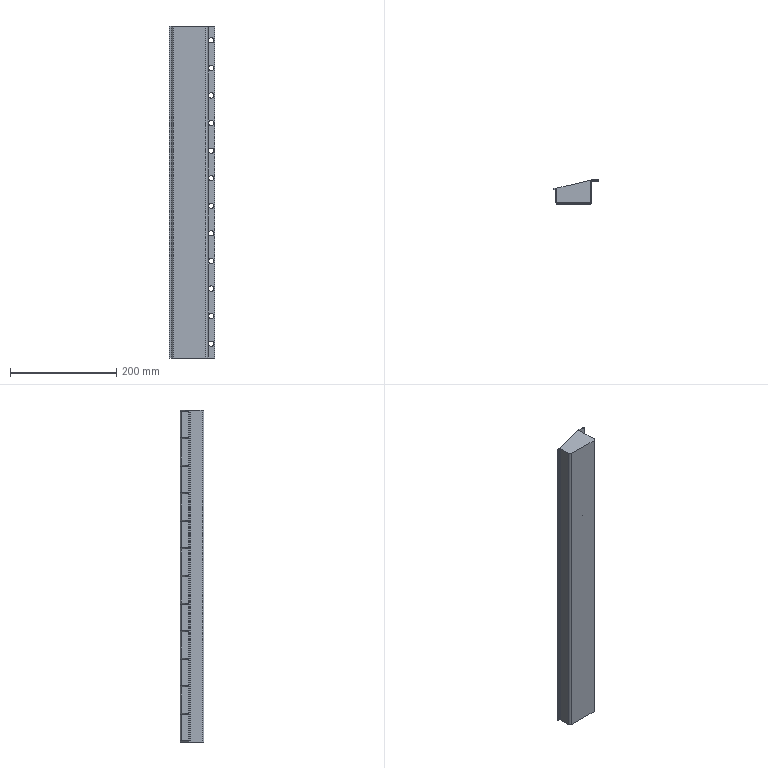Part | STEP file | Storage insert | 1 solid | 138 faces | box 86 x 45 x 626 mm | volume 245916 mm3 | plane 84 | cylinder 54 | commonest cylinder face diameters 3 x26 10 x24 7 x3 6 x1